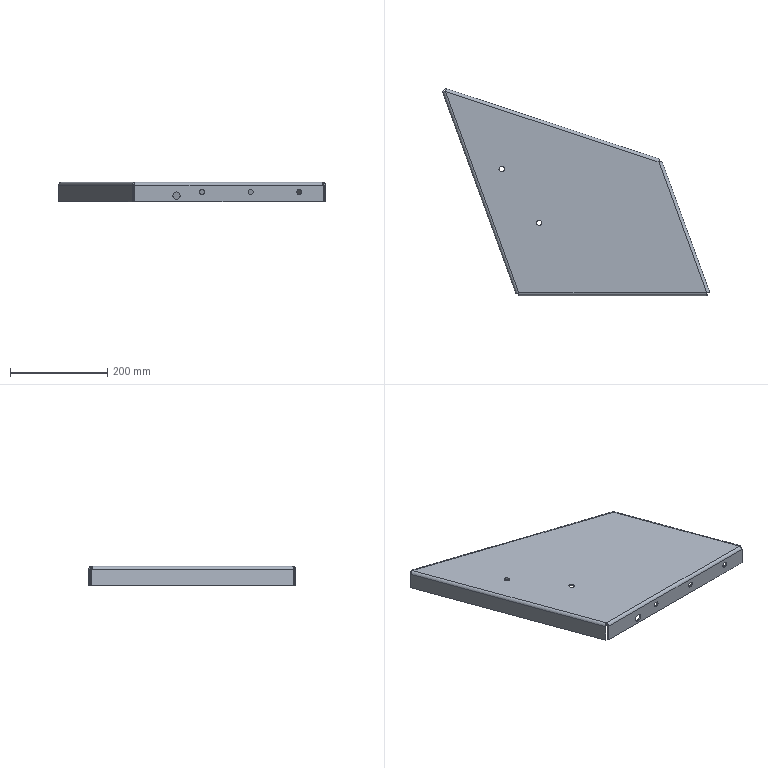Part | SolidWorks | features BaseBody 1 | 1 solid | 56 faces | box 550.856 x 426.984 x 40 mm | volume 590475 mm3 | plane 36 | cylinder 20 | commonest cylinder face diameters 11 x10 6 x4 12 x4 15 x2